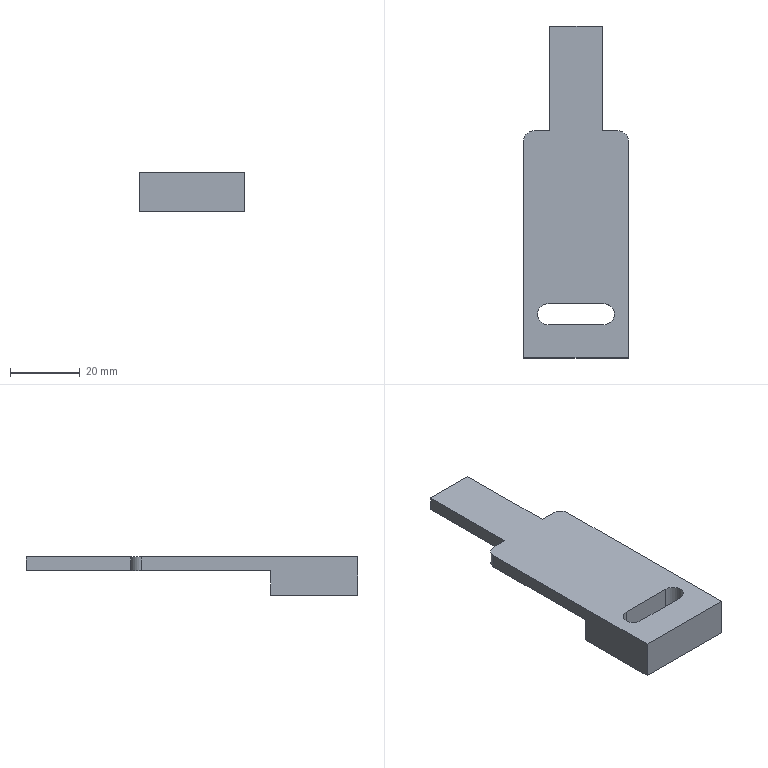Part | SolidWorks | features ICE 2, Extrusion 1, Fillet 1 | 1 solid | 19 faces | box 30 x 95 x 11 mm | volume 13468 mm3 | plane 14 | cylinder 5 | commonest cylinder face diameters 6 x5
STEP:
#1=CARTESIAN_POINT('',(-8.,15.5,11.));
#2=VERTEX_POINT('',#1);
#3=CARTESIAN_POINT('',(-11.,12.5,11.));
#4=VERTEX_POINT('',#3);
#5=CARTESIAN_POINT('',(-8.,12.5,11.));
#6=DIRECTION('',(0.,0.,1.));
#7=DIRECTION('',(1.,0.,0.));
#8=AXIS2_PLACEMENT_3D('',#5,#6,#7);
#9=CIRCLE('',#8,3.);
#10=EDGE_CURVE('',#2,#4,#9,.T.);
#11=ORIENTED_EDGE('',*,*,#10,.T.);
#12=CARTESIAN_POINT('',(-11.,12.5,0.));
#13=VERTEX_POINT('',#12);
#14=CARTESIAN_POINT('',(-11.,12.5,7.));
#15=DIRECTION('',(0.,0.,-1.));
#16=VECTOR('',#15,1000.);
#17=LINE('',#14,#16);
#18=EDGE_CURVE('',#4,#13,#17,.T.);
#19=ORIENTED_EDGE('',*,*,#18,.T.);
#20=CARTESIAN_POINT('',(-8.,15.5,0.));
#21=VERTEX_POINT('',#20);
#22=CARTESIAN_POINT('',(-8.,12.5,0.));
#23=DIRECTION('',(0.,0.,1.));
#24=DIRECTION('',(1.,0.,0.));
#25=AXIS2_PLACEMENT_3D('',#22,#23,#24);
#26=CIRCLE('',#25,3.);
#27=EDGE_CURVE('',#21,#13,#26,.T.);
#28=ORIENTED_EDGE('',*,*,#27,.F.);
#29=CARTESIAN_POINT('',(-8.,15.5,7.));
#30=DIRECTION('',(0.,0.,-1.));
#31=VECTOR('',#30,1000.);
#32=LINE('',#29,#31);
#33=EDGE_CURVE('',#2,#21,#32,.T.);
#34=ORIENTED_EDGE('',*,*,#33,.F.);
#35=EDGE_LOOP('',(#11,#19,#28,#34));
#36=FACE_OUTER_BOUND('',#35,.T.);
#37=CARTESIAN_POINT('',(-8.,12.5,7.));
#38=DIRECTION('',(0.,0.,-1.));
#39=DIRECTION('',(-1.,0.,0.));
#40=AXIS2_PLACEMENT_3D('',#37,#38,#39);
#41=CYLINDRICAL_SURFACE('',#40,3.);
#42=ADVANCED_FACE('',(#36),#41,.F.);
#43=CARTESIAN_POINT('',(12.,65.,7.));
#44=VERTEX_POINT('',#43);
#45=CARTESIAN_POINT('',(7.5,65.,7.));
#46=VERTEX_POINT('',#45);
#47=CARTESIAN_POINT('',(-15.,65.,7.));
#48=DIRECTION('',(-1.,0.,0.));
#49=VECTOR('',#48,1000.);
#50=LINE('',#47,#49);
#51=EDGE_CURVE('',#44,#46,#50,.T.);
#52=ORIENTED_EDGE('',*,*,#51,.T.);
#53=CARTESIAN_POINT('',(7.5,65.,11.));
#54=VERTEX_POINT('',#53);
#55=CARTESIAN_POINT('',(7.5,65.,-26.541));
#56=DIRECTION('',(0.,0.,1.));
#57=VECTOR('',#56,1000.);
#58=LINE('',#55,#57);
#59=EDGE_CURVE('',#46,#54,#58,.T.);
#60=ORIENTED_EDGE('',*,*,#59,.T.);
#61=CARTESIAN_POINT('',(12.,65.,11.));
#62=VERTEX_POINT('',#61);
#63=CARTESIAN_POINT('',(-15.,65.,11.));
#64=DIRECTION('',(-1.,0.,0.));
#65=VECTOR('',#64,1000.);
#66=LINE('',#63,#65);
#67=EDGE_CURVE('',#62,#54,#66,.T.);
#68=ORIENTED_EDGE('',*,*,#67,.F.);
#69=CARTESIAN_POINT('',(12.,65.,11.));
#70=DIRECTION('',(0.,0.,-1.));
#71=VECTOR('',#70,1000.);
#72=LINE('',#69,#71);
#73=EDGE_CURVE('',#62,#44,#72,.T.);
#74=ORIENTED_EDGE('',*,*,#73,.T.);
#75=EDGE_LOOP('',(#52,#60,#68,#74));
#76=FACE_OUTER_BOUND('',#75,.T.);
#77=CARTESIAN_POINT('',(-15.,65.,11.));
#78=DIRECTION('',(0.,-1.,0.));
#79=DIRECTION('',(0.,0.,-1.));
#80=AXIS2_PLACEMENT_3D('',#77,#78,#79);
#81=PLANE('',#80);
#82=ADVANCED_FACE('',(#76),#81,.F.);
#83=CARTESIAN_POINT('',(15.,0.,0.));
#84=VERTEX_POINT('',#83);
#85=CARTESIAN_POINT('',(15.,25.,0.));
#86=VERTEX_POINT('',#85);
#87=CARTESIAN_POINT('',(15.,25.,0.));
#88=DIRECTION('',(0.,1.,0.));
#89=VECTOR('',#88,1000.);
#90=LINE('',#87,#89);
#91=EDGE_CURVE('',#84,#86,#90,.T.);
#92=ORIENTED_EDGE('',*,*,#91,.F.);
#93=CARTESIAN_POINT('',(-15.,0.,0.));
#94=VERTEX_POINT('',#93);
#95=CARTESIAN_POINT('',(0.,0.,0.));
#96=DIRECTION('',(1.,0.,0.));
#97=VECTOR('',#96,1000.);
#98=LINE('',#95,#97);
#99=EDGE_CURVE('',#94,#84,#98,.T.);
#100=ORIENTED_EDGE('',*,*,#99,.F.);
#101=CARTESIAN_POINT('',(-15.,25.,0.));
#102=VERTEX_POINT('',#101);
#103=CARTESIAN_POINT('',(-15.,0.,0.));
#104=DIRECTION('',(0.,-1.,0.));
#105=VECTOR('',#104,1000.);
#106=LINE('',#103,#105);
#107=EDGE_CURVE('',#102,#94,#106,.T.);
#108=ORIENTED_EDGE('',*,*,#107,.F.);
#109=CARTESIAN_POINT('',(-15.,25.,0.));
#110=DIRECTION('',(-1.,0.,0.));
#111=VECTOR('',#110,1000.);
#112=LINE('',#109,#111);
#113=EDGE_CURVE('',#86,#102,#112,.T.);
#114=ORIENTED_EDGE('',*,*,#113,.F.);
#115=EDGE_LOOP('',(#92,#100,#108,#114));
#116=FACE_OUTER_BOUND('',#115,.T.);
#117=CARTESIAN_POINT('',(8.,15.5,0.));
#118=VERTEX_POINT('',#117);
#119=CARTESIAN_POINT('',(-8.,15.5,0.));
#120=DIRECTION('',(-1.,0.,0.));
#121=VECTOR('',#120,1000.);
#122=LINE('',#119,#121);
#123=EDGE_CURVE('',#118,#21,#122,.T.);
#124=ORIENTED_EDGE('',*,*,#123,.T.);
#125=ORIENTED_EDGE('',*,*,#27,.T.);
#126=CARTESIAN_POINT('',(-8.,9.5,0.));
#127=VERTEX_POINT('',#126);
#128=CARTESIAN_POINT('',(-8.,12.5,0.));
#129=DIRECTION('',(0.,0.,1.));
#130=DIRECTION('',(1.,0.,0.));
#131=AXIS2_PLACEMENT_3D('',#128,#129,#130);
#132=CIRCLE('',#131,3.);
#133=EDGE_CURVE('',#13,#127,#132,.T.);
#134=ORIENTED_EDGE('',*,*,#133,.T.);
#135=CARTESIAN_POINT('',(8.,9.5,0.));
#136=VERTEX_POINT('',#135);
#137=CARTESIAN_POINT('',(-8.,9.5,0.));
#138=DIRECTION('',(1.,0.,0.));
#139=VECTOR('',#138,1000.);
#140=LINE('',#137,#139);
#141=EDGE_CURVE('',#127,#136,#140,.T.);
#142=ORIENTED_EDGE('',*,*,#141,.T.);
#143=CARTESIAN_POINT('',(8.,12.5,0.));
#144=DIRECTION('',(0.,0.,1.));
#145=DIRECTION('',(1.,0.,0.));
#146=AXIS2_PLACEMENT_3D('',#143,#144,#145);
#147=CIRCLE('',#146,3.);
#148=EDGE_CURVE('',#136,#118,#147,.T.);
#149=ORIENTED_EDGE('',*,*,#148,.T.);
#150=EDGE_LOOP('',(#124,#125,#134,#142,#149));
#151=FACE_BOUND('',#150,.T.);
#152=CARTESIAN_POINT('',(0.,0.,0.));
#153=DIRECTION('',(0.,0.,-1.));
#154=DIRECTION('',(-1.,0.,0.));
#155=AXIS2_PLACEMENT_3D('',#152,#153,#154);
#156=PLANE('',#155);
#157=ADVANCED_FACE('',(#116,#151),#156,.T.);
#158=CARTESIAN_POINT('',(15.,25.,7.));
#159=VERTEX_POINT('',#158);
#160=CARTESIAN_POINT('',(15.,62.,7.));
#161=VERTEX_POINT('',#160);
#162=CARTESIAN_POINT('',(15.,0.,7.));
#163=DIRECTION('',(0.,1.,0.));
#164=VECTOR('',#163,1000.);
#165=LINE('',#162,#164);
#166=EDGE_CURVE('',#159,#161,#165,.T.);
#167=ORIENTED_EDGE('',*,*,#166,.T.);
#168=CARTESIAN_POINT('',(15.,62.,11.));
#169=VERTEX_POINT('',#168);
#170=CARTESIAN_POINT('',(15.,62.,7.));
#171=DIRECTION('',(0.,0.,1.));
#172=VECTOR('',#171,1000.);
#173=LINE('',#170,#172);
#174=EDGE_CURVE('',#161,#169,#173,.T.);
#175=ORIENTED_EDGE('',*,*,#174,.T.);
#176=CARTESIAN_POINT('',(15.,0.,11.));
#177=VERTEX_POINT('',#176);
#178=CARTESIAN_POINT('',(15.,0.,11.));
#179=DIRECTION('',(0.,1.,0.));
#180=VECTOR('',#179,1000.);
#181=LINE('',#178,#180);
#182=EDGE_CURVE('',#177,#169,#181,.T.);
#183=ORIENTED_EDGE('',*,*,#182,.F.);
#184=CARTESIAN_POINT('',(15.,0.,7.));
#185=DIRECTION('',(0.,0.,-1.));
#186=VECTOR('',#185,1000.);
#187=LINE('',#184,#186);
#188=EDGE_CURVE('',#177,#84,#187,.T.);
#189=ORIENTED_EDGE('',*,*,#188,.T.);
#190=ORIENTED_EDGE('',*,*,#91,.T.);
#191=CARTESIAN_POINT('',(15.,25.,7.));
#192=DIRECTION('',(0.,0.,-1.));
#193=VECTOR('',#192,1000.);
#194=LINE('',#191,#193);
#195=EDGE_CURVE('',#159,#86,#194,.T.);
#196=ORIENTED_EDGE('',*,*,#195,.F.);
#197=EDGE_LOOP('',(#167,#175,#183,#189,#190,#196));
#198=FACE_OUTER_BOUND('',#197,.T.);
#199=CARTESIAN_POINT('',(15.,25.,7.));
#200=DIRECTION('',(-1.,0.,0.));
#201=DIRECTION('',(0.,0.,1.));
#202=AXIS2_PLACEMENT_3D('',#199,#200,#201);
#203=PLANE('',#202);
#204=ADVANCED_FACE('',(#198),#203,.F.);
#205=ORIENTED_EDGE('',*,*,#113,.T.);
#206=CARTESIAN_POINT('',(-15.,25.,7.));
#207=VERTEX_POINT('',#206);
#208=CARTESIAN_POINT('',(-15.,25.,7.));
#209=DIRECTION('',(0.,0.,-1.));
#210=VECTOR('',#209,1000.);
#211=LINE('',#208,#210);
#212=EDGE_CURVE('',#207,#102,#211,.T.);
#213=ORIENTED_EDGE('',*,*,#212,.F.);
#214=CARTESIAN_POINT('',(-15.,25.,7.));
#215=DIRECTION('',(-1.,0.,0.));
#216=VECTOR('',#215,1000.);
#217=LINE('',#214,#216);
#218=EDGE_CURVE('',#159,#207,#217,.T.);
#219=ORIENTED_EDGE('',*,*,#218,.F.);
#220=ORIENTED_EDGE('',*,*,#195,.T.);
#221=EDGE_LOOP('',(#205,#213,#219,#220));
#222=FACE_OUTER_BOUND('',#221,.T.);
#223=CARTESIAN_POINT('',(-15.,25.,7.));
#224=DIRECTION('',(0.,-1.,0.));
#225=DIRECTION('',(1.,0.,0.));
#226=AXIS2_PLACEMENT_3D('',#223,#224,#225);
#227=PLANE('',#226);
#228=ADVANCED_FACE('',(#222),#227,.F.);
#229=CARTESIAN_POINT('',(-15.,62.,11.));
#230=VERTEX_POINT('',#229);
#231=CARTESIAN_POINT('',(-15.,0.,11.));
#232=VERTEX_POINT('',#231);
#233=CARTESIAN_POINT('',(-15.,0.,11.));
#234=DIRECTION('',(0.,-1.,0.));
#235=VECTOR('',#234,1000.);
#236=LINE('',#233,#235);
#237=EDGE_CURVE('',#230,#232,#236,.T.);
#238=ORIENTED_EDGE('',*,*,#237,.F.);
#239=CARTESIAN_POINT('',(-15.,62.,7.));
#240=VERTEX_POINT('',#239);
#241=CARTESIAN_POINT('',(-15.,62.,7.));
#242=DIRECTION('',(0.,0.,-1.));
#243=VECTOR('',#242,1000.);
#244=LINE('',#241,#243);
#245=EDGE_CURVE('',#230,#240,#244,.T.);
#246=ORIENTED_EDGE('',*,*,#245,.T.);
#247=CARTESIAN_POINT('',(-15.,0.,7.));
#248=DIRECTION('',(0.,-1.,0.));
#249=VECTOR('',#248,1000.);
#250=LINE('',#247,#249);
#251=EDGE_CURVE('',#240,#207,#250,.T.);
#252=ORIENTED_EDGE('',*,*,#251,.T.);
#253=ORIENTED_EDGE('',*,*,#212,.T.);
#254=ORIENTED_EDGE('',*,*,#107,.T.);
#255=CARTESIAN_POINT('',(-15.,0.,7.));
#256=DIRECTION('',(0.,0.,-1.));
#257=VECTOR('',#256,1000.);
#258=LINE('',#255,#257);
#259=EDGE_CURVE('',#232,#94,#258,.T.);
#260=ORIENTED_EDGE('',*,*,#259,.F.);
#261=EDGE_LOOP('',(#238,#246,#252,#253,#254,#260));
#262=FACE_OUTER_BOUND('',#261,.T.);
#263=CARTESIAN_POINT('',(-15.,0.,7.));
#264=DIRECTION('',(1.,0.,0.));
#265=DIRECTION('',(0.,1.,0.));
#266=AXIS2_PLACEMENT_3D('',#263,#264,#265);
#267=PLANE('',#266);
#268=ADVANCED_FACE('',(#262),#267,.F.);
#269=ORIENTED_EDGE('',*,*,#99,.T.);
#270=ORIENTED_EDGE('',*,*,#188,.F.);
#271=CARTESIAN_POINT('',(-15.,0.,11.));
#272=DIRECTION('',(1.,0.,0.));
#273=VECTOR('',#272,1000.);
#274=LINE('',#271,#273);
#275=EDGE_CURVE('',#232,#177,#274,.T.);
#276=ORIENTED_EDGE('',*,*,#275,.F.);
#277=ORIENTED_EDGE('',*,*,#259,.T.);
#278=EDGE_LOOP('',(#269,#270,#276,#277));
#279=FACE_OUTER_BOUND('',#278,.T.);
#280=CARTESIAN_POINT('',(0.,0.,7.));
#281=DIRECTION('',(0.,1.,0.));
#282=DIRECTION('',(-1.,0.,0.));
#283=AXIS2_PLACEMENT_3D('',#280,#281,#282);
#284=PLANE('',#283);
#285=ADVANCED_FACE('',(#279),#284,.F.);
#286=ORIENTED_EDGE('',*,*,#18,.F.);
#287=CARTESIAN_POINT('',(-8.,9.5,11.));
#288=VERTEX_POINT('',#287);
#289=CARTESIAN_POINT('',(-8.,12.5,11.));
#290=DIRECTION('',(0.,0.,1.));
#291=DIRECTION('',(1.,0.,0.));
#292=AXIS2_PLACEMENT_3D('',#289,#290,#291);
#293=CIRCLE('',#292,3.);
#294=EDGE_CURVE('',#4,#288,#293,.T.);
#295=ORIENTED_EDGE('',*,*,#294,.T.);
#296=CARTESIAN_POINT('',(-8.,9.5,7.));
#297=DIRECTION('',(0.,0.,-1.));
#298=VECTOR('',#297,1000.);
#299=LINE('',#296,#298);
#300=EDGE_CURVE('',#288,#127,#299,.T.);
#301=ORIENTED_EDGE('',*,*,#300,.T.);
#302=ORIENTED_EDGE('',*,*,#133,.F.);
#303=EDGE_LOOP('',(#286,#295,#301,#302));
#304=FACE_OUTER_BOUND('',#303,.T.);
#305=CARTESIAN_POINT('',(-8.,12.5,7.));
#306=DIRECTION('',(0.,0.,-1.));
#307=DIRECTION('',(-1.,0.,0.));
#308=AXIS2_PLACEMENT_3D('',#305,#306,#307);
#309=CYLINDRICAL_SURFACE('',#308,3.);
#310=ADVANCED_FACE('',(#304),#309,.F.);
#311=ORIENTED_EDGE('',*,*,#141,.F.);
#312=ORIENTED_EDGE('',*,*,#300,.F.);
#313=CARTESIAN_POINT('',(8.,9.5,11.));
#314=VERTEX_POINT('',#313);
#315=CARTESIAN_POINT('',(-8.,9.5,11.));
#316=DIRECTION('',(1.,0.,0.));
#317=VECTOR('',#316,1000.);
#318=LINE('',#315,#317);
#319=EDGE_CURVE('',#288,#314,#318,.T.);
#320=ORIENTED_EDGE('',*,*,#319,.T.);
#321=CARTESIAN_POINT('',(8.,9.5,7.));
#322=DIRECTION('',(0.,0.,-1.));
#323=VECTOR('',#322,1000.);
#324=LINE('',#321,#323);
#325=EDGE_CURVE('',#314,#136,#324,.T.);
#326=ORIENTED_EDGE('',*,*,#325,.T.);
#327=EDGE_LOOP('',(#311,#312,#320,#326));
#328=FACE_OUTER_BOUND('',#327,.T.);
#329=CARTESIAN_POINT('',(-8.,9.5,7.));
#330=DIRECTION('',(0.,1.,0.));
#331=DIRECTION('',(0.,0.,1.));
#332=AXIS2_PLACEMENT_3D('',#329,#330,#331);
#333=PLANE('',#332);
#334=ADVANCED_FACE('',(#328),#333,.T.);
#335=ORIENTED_EDGE('',*,*,#148,.F.);
#336=ORIENTED_EDGE('',*,*,#325,.F.);
#337=CARTESIAN_POINT('',(8.,15.5,11.));
#338=VERTEX_POINT('',#337);
#339=CARTESIAN_POINT('',(8.,12.5,11.));
#340=DIRECTION('',(0.,0.,1.));
#341=DIRECTION('',(1.,0.,0.));
#342=AXIS2_PLACEMENT_3D('',#339,#340,#341);
#343=CIRCLE('',#342,3.);
#344=EDGE_CURVE('',#314,#338,#343,.T.);
#345=ORIENTED_EDGE('',*,*,#344,.T.);
#346=CARTESIAN_POINT('',(8.,15.5,7.));
#347=DIRECTION('',(0.,0.,-1.));
#348=VECTOR('',#347,1000.);
#349=LINE('',#346,#348);
#350=EDGE_CURVE('',#338,#118,#349,.T.);
#351=ORIENTED_EDGE('',*,*,#350,.T.);
#352=EDGE_LOOP('',(#335,#336,#345,#351));
#353=FACE_OUTER_BOUND('',#352,.T.);
#354=CARTESIAN_POINT('',(8.,12.5,7.));
#355=DIRECTION('',(0.,0.,-1.));
#356=DIRECTION('',(-1.,0.,0.));
#357=AXIS2_PLACEMENT_3D('',#354,#355,#356);
#358=CYLINDRICAL_SURFACE('',#357,3.);
#359=ADVANCED_FACE('',(#353),#358,.F.);
#360=ORIENTED_EDGE('',*,*,#123,.F.);
#361=ORIENTED_EDGE('',*,*,#350,.F.);
#362=CARTESIAN_POINT('',(8.,15.5,11.));
#363=DIRECTION('',(-1.,0.,0.));
#364=VECTOR('',#363,1000.);
#365=LINE('',#362,#364);
#366=EDGE_CURVE('',#338,#2,#365,.T.);
#367=ORIENTED_EDGE('',*,*,#366,.T.);
#368=ORIENTED_EDGE('',*,*,#33,.T.);
#369=EDGE_LOOP('',(#360,#361,#367,#368));
#370=FACE_OUTER_BOUND('',#369,.T.);
#371=CARTESIAN_POINT('',(-8.,15.5,7.));
#372=DIRECTION('',(0.,-1.,0.));
#373=DIRECTION('',(0.,0.,-1.));
#374=AXIS2_PLACEMENT_3D('',#371,#372,#373);
#375=PLANE('',#374);
#376=ADVANCED_FACE('',(#370),#375,.T.);
#377=ORIENTED_EDGE('',*,*,#182,.T.);
#378=CARTESIAN_POINT('',(12.,62.,11.));
#379=DIRECTION('',(0.,0.,1.));
#380=DIRECTION('',(-1.,0.,0.));
#381=AXIS2_PLACEMENT_3D('',#378,#379,#380);
#382=CIRCLE('',#381,3.);
#383=EDGE_CURVE('',#169,#62,#382,.T.);
#384=ORIENTED_EDGE('',*,*,#383,.T.);
#385=ORIENTED_EDGE('',*,*,#67,.T.);
#386=CARTESIAN_POINT('',(7.5,95.,11.));
#387=VERTEX_POINT('',#386);
#388=CARTESIAN_POINT('',(7.5,95.,11.));
#389=DIRECTION('',(0.,1.,0.));
#390=VECTOR('',#389,1000.);
#391=LINE('',#388,#390);
#392=EDGE_CURVE('',#54,#387,#391,.T.);
#393=ORIENTED_EDGE('',*,*,#392,.T.);
#394=CARTESIAN_POINT('',(-7.5,95.,11.));
#395=VERTEX_POINT('',#394);
#396=CARTESIAN_POINT('',(-7.5,95.,11.));
#397=DIRECTION('',(-1.,0.,0.));
#398=VECTOR('',#397,1000.);
#399=LINE('',#396,#398);
#400=EDGE_CURVE('',#387,#395,#399,.T.);
#401=ORIENTED_EDGE('',*,*,#400,.T.);
#402=CARTESIAN_POINT('',(-7.5,65.,11.));
#403=VERTEX_POINT('',#402);
#404=CARTESIAN_POINT('',(-7.5,65.,11.));
#405=DIRECTION('',(0.,-1.,0.));
#406=VECTOR('',#405,1000.);
#407=LINE('',#404,#406);
#408=EDGE_CURVE('',#395,#403,#407,.T.);
#409=ORIENTED_EDGE('',*,*,#408,.T.);
#410=CARTESIAN_POINT('',(-12.,65.,11.));
#411=VERTEX_POINT('',#410);
#412=CARTESIAN_POINT('',(-15.,65.,11.));
#413=DIRECTION('',(-1.,0.,0.));
#414=VECTOR('',#413,1000.);
#415=LINE('',#412,#414);
#416=EDGE_CURVE('',#403,#411,#415,.T.);
#417=ORIENTED_EDGE('',*,*,#416,.T.);
#418=CARTESIAN_POINT('',(-12.,62.,11.));
#419=DIRECTION('',(0.,0.,1.));
#420=DIRECTION('',(-1.,0.,0.));
#421=AXIS2_PLACEMENT_3D('',#418,#419,#420);
#422=CIRCLE('',#421,3.);
#423=EDGE_CURVE('',#411,#230,#422,.T.);
#424=ORIENTED_EDGE('',*,*,#423,.T.);
#425=ORIENTED_EDGE('',*,*,#237,.T.);
#426=ORIENTED_EDGE('',*,*,#275,.T.);
#427=EDGE_LOOP('',(#377,#384,#385,#393,#401,#409,#417,#424,#425,#426));
#428=FACE_OUTER_BOUND('',#427,.T.);
#429=ORIENTED_EDGE('',*,*,#344,.F.);
#430=ORIENTED_EDGE('',*,*,#319,.F.);
#431=ORIENTED_EDGE('',*,*,#294,.F.);
#432=ORIENTED_EDGE('',*,*,#10,.F.);
#433=ORIENTED_EDGE('',*,*,#366,.F.);
#434=EDGE_LOOP('',(#429,#430,#431,#432,#433));
#435=FACE_BOUND('',#434,.T.);
#436=CARTESIAN_POINT('',(0.,0.,11.));
#437=DIRECTION('',(0.,0.,-1.));
#438=DIRECTION('',(-1.,0.,0.));
#439=AXIS2_PLACEMENT_3D('',#436,#437,#438);
#440=PLANE('',#439);
#441=ADVANCED_FACE('',(#428,#435),#440,.F.);
#442=ORIENTED_EDGE('',*,*,#51,.F.);
#443=CARTESIAN_POINT('',(12.,62.,7.));
#444=DIRECTION('',(0.,0.,-1.));
#445=DIRECTION('',(-1.,0.,0.));
#446=AXIS2_PLACEMENT_3D('',#443,#444,#445);
#447=CIRCLE('',#446,3.);
#448=EDGE_CURVE('',#44,#161,#447,.T.);
#449=ORIENTED_EDGE('',*,*,#448,.T.);
#450=ORIENTED_EDGE('',*,*,#166,.F.);
#451=ORIENTED_EDGE('',*,*,#218,.T.);
#452=ORIENTED_EDGE('',*,*,#251,.F.);
#453=CARTESIAN_POINT('',(-12.,65.,7.));
#454=VERTEX_POINT('',#453);
#455=CARTESIAN_POINT('',(-12.,62.,7.));
#456=DIRECTION('',(0.,0.,-1.));
#457=DIRECTION('',(-1.,0.,0.));
#458=AXIS2_PLACEMENT_3D('',#455,#456,#457);
#459=CIRCLE('',#458,3.);
#460=EDGE_CURVE('',#240,#454,#459,.T.);
#461=ORIENTED_EDGE('',*,*,#460,.T.);
#462=CARTESIAN_POINT('',(-7.5,65.,7.));
#463=VERTEX_POINT('',#462);
#464=CARTESIAN_POINT('',(-15.,65.,7.));
#465=DIRECTION('',(-1.,0.,0.));
#466=VECTOR('',#465,1000.);
#467=LINE('',#464,#466);
#468=EDGE_CURVE('',#463,#454,#467,.T.);
#469=ORIENTED_EDGE('',*,*,#468,.F.);
#470=CARTESIAN_POINT('',(-7.5,95.,7.));
#471=VERTEX_POINT('',#470);
#472=CARTESIAN_POINT('',(-7.5,65.,7.));
#473=DIRECTION('',(0.,-1.,0.));
#474=VECTOR('',#473,1000.);
#475=LINE('',#472,#474);
#476=EDGE_CURVE('',#471,#463,#475,.T.);
#477=ORIENTED_EDGE('',*,*,#476,.F.);
#478=CARTESIAN_POINT('',(7.5,95.,7.));
#479=VERTEX_POINT('',#478);
#480=CARTESIAN_POINT('',(-7.5,95.,7.));
#481=DIRECTION('',(-1.,0.,0.));
#482=VECTOR('',#481,1000.);
#483=LINE('',#480,#482);
#484=EDGE_CURVE('',#479,#471,#483,.T.);
#485=ORIENTED_EDGE('',*,*,#484,.F.);
#486=CARTESIAN_POINT('',(7.5,95.,7.));
#487=DIRECTION('',(0.,1.,0.));
#488=VECTOR('',#487,1000.);
#489=LINE('',#486,#488);
#490=EDGE_CURVE('',#46,#479,#489,.T.);
#491=ORIENTED_EDGE('',*,*,#490,.F.);
#492=EDGE_LOOP('',(#442,#449,#450,#451,#452,#461,#469,#477,#485,#491));
#493=FACE_OUTER_BOUND('',#492,.T.);
#494=CARTESIAN_POINT('',(0.,0.,7.));
#495=DIRECTION('',(0.,0.,-1.));
#496=DIRECTION('',(-1.,0.,0.));
#497=AXIS2_PLACEMENT_3D('',#494,#495,#496);
#498=PLANE('',#497);
#499=ADVANCED_FACE('',(#493),#498,.T.);
#500=ORIENTED_EDGE('',*,*,#416,.F.);
#501=CARTESIAN_POINT('',(-7.5,65.,-26.541));
#502=DIRECTION('',(0.,0.,1.));
#503=VECTOR('',#502,1000.);
#504=LINE('',#501,#503);
#505=EDGE_CURVE('',#463,#403,#504,.T.);
#506=ORIENTED_EDGE('',*,*,#505,.F.);
#507=ORIENTED_EDGE('',*,*,#468,.T.);
#508=CARTESIAN_POINT('',(-12.,65.,11.));
#509=DIRECTION('',(0.,0.,1.));
#510=VECTOR('',#509,1000.);
#511=LINE('',#508,#510);
#512=EDGE_CURVE('',#454,#411,#511,.T.);
#513=ORIENTED_EDGE('',*,*,#512,.T.);
#514=EDGE_LOOP('',(#500,#506,#507,#513));
#515=FACE_OUTER_BOUND('',#514,.T.);
#516=CARTESIAN_POINT('',(-15.,65.,11.));
#517=DIRECTION('',(0.,-1.,0.));
#518=DIRECTION('',(0.,0.,-1.));
#519=AXIS2_PLACEMENT_3D('',#516,#517,#518);
#520=PLANE('',#519);
#521=ADVANCED_FACE('',(#515),#520,.F.);
#522=ORIENTED_EDGE('',*,*,#383,.F.);
#523=ORIENTED_EDGE('',*,*,#174,.F.);
#524=ORIENTED_EDGE('',*,*,#448,.F.);
#525=ORIENTED_EDGE('',*,*,#73,.F.);
#526=EDGE_LOOP('',(#522,#523,#524,#525));
#527=FACE_OUTER_BOUND('',#526,.T.);
#528=CARTESIAN_POINT('',(12.,62.,11.));
#529=DIRECTION('',(0.,0.,-1.));
#530=DIRECTION('',(-1.,0.,0.));
#531=AXIS2_PLACEMENT_3D('',#528,#529,#530);
#532=CYLINDRICAL_SURFACE('',#531,3.);
#533=ADVANCED_FACE('',(#527),#532,.T.);
#534=ORIENTED_EDGE('',*,*,#423,.F.);
#535=ORIENTED_EDGE('',*,*,#512,.F.);
#536=ORIENTED_EDGE('',*,*,#460,.F.);
#537=ORIENTED_EDGE('',*,*,#245,.F.);
#538=EDGE_LOOP('',(#534,#535,#536,#537));
#539=FACE_OUTER_BOUND('',#538,.T.);
#540=CARTESIAN_POINT('',(-12.,62.,7.));
#541=DIRECTION('',(0.,0.,-1.));
#542=DIRECTION('',(-1.,0.,0.));
#543=AXIS2_PLACEMENT_3D('',#540,#541,#542);
#544=CYLINDRICAL_SURFACE('',#543,3.);
#545=ADVANCED_FACE('',(#539),#544,.T.);
#546=ORIENTED_EDGE('',*,*,#59,.F.);
#547=ORIENTED_EDGE('',*,*,#490,.T.);
#548=CARTESIAN_POINT('',(7.5,95.,-26.541));
#549=DIRECTION('',(0.,0.,1.));
#550=VECTOR('',#549,1000.);
#551=LINE('',#548,#550);
#552=EDGE_CURVE('',#479,#387,#551,.T.);
#553=ORIENTED_EDGE('',*,*,#552,.T.);
#554=ORIENTED_EDGE('',*,*,#392,.F.);
#555=EDGE_LOOP('',(#546,#547,#553,#554));
#556=FACE_OUTER_BOUND('',#555,.T.);
#557=CARTESIAN_POINT('',(7.5,95.,-26.541));
#558=DIRECTION('',(1.,0.,0.));
#559=DIRECTION('',(0.,1.,0.));
#560=AXIS2_PLACEMENT_3D('',#557,#558,#559);
#561=PLANE('',#560);
#562=ADVANCED_FACE('',(#556),#561,.T.);
#563=ORIENTED_EDGE('',*,*,#552,.F.);
#564=ORIENTED_EDGE('',*,*,#484,.T.);
#565=CARTESIAN_POINT('',(-7.5,95.,-26.541));
#566=DIRECTION('',(0.,0.,1.));
#567=VECTOR('',#566,1000.);
#568=LINE('',#565,#567);
#569=EDGE_CURVE('',#471,#395,#568,.T.);
#570=ORIENTED_EDGE('',*,*,#569,.T.);
#571=ORIENTED_EDGE('',*,*,#400,.F.);
#572=EDGE_LOOP('',(#563,#564,#570,#571));
#573=FACE_OUTER_BOUND('',#572,.T.);
#574=CARTESIAN_POINT('',(-7.5,95.,-26.541));
#575=DIRECTION('',(0.,1.,0.));
#576=DIRECTION('',(0.,0.,1.));
#577=AXIS2_PLACEMENT_3D('',#574,#575,#576);
#578=PLANE('',#577);
#579=ADVANCED_FACE('',(#573),#578,.T.);
#580=ORIENTED_EDGE('',*,*,#569,.F.);
#581=ORIENTED_EDGE('',*,*,#476,.T.);
#582=ORIENTED_EDGE('',*,*,#505,.T.);
#583=ORIENTED_EDGE('',*,*,#408,.F.);
#584=EDGE_LOOP('',(#580,#581,#582,#583));
#585=FACE_OUTER_BOUND('',#584,.T.);
#586=CARTESIAN_POINT('',(-7.5,65.,-26.541));
#587=DIRECTION('',(-1.,0.,0.));
#588=DIRECTION('',(0.,-1.,0.));
#589=AXIS2_PLACEMENT_3D('',#586,#587,#588);
#590=PLANE('',#589);
#591=ADVANCED_FACE('',(#585),#590,.T.);
#592=CLOSED_SHELL('',(#42,#82,#157,#204,#228,#268,#285,#310,#334,#359,#376,#441,#499,#521,#533,#545,#562,#579,#591));
#593=MANIFOLD_SOLID_BREP('',#592);
#594=CARTESIAN_POINT('',(0.,0.,0.));
#595=DIRECTION('',(0.,0.,1.));
#596=DIRECTION('',(1.,0.,0.));
#597=AXIS2_PLACEMENT_3D('',#594,#595,#596);
#598=(LENGTH_UNIT()NAMED_UNIT(*)SI_UNIT(.MILLI.,.METRE.));
#599=UNCERTAINTY_MEASURE_WITH_UNIT(LENGTH_MEASURE(0.00001),#598,'','');
#600=(NAMED_UNIT(*)PLANE_ANGLE_UNIT()SI_UNIT($,.RADIAN.));
#601=(NAMED_UNIT(*)SI_UNIT($,.STERADIAN.)SOLID_ANGLE_UNIT());
#602=(GEOMETRIC_REPRESENTATION_CONTEXT(3)GLOBAL_UNCERTAINTY_ASSIGNED_CONTEXT((#599))GLOBAL_UNIT_ASSIGNED_CONTEXT((#598,#600,#601))REPRESENTATION_CONTEXT('',''));
#603=ADVANCED_BREP_SHAPE_REPRESENTATION('',(#593,#597),#602);